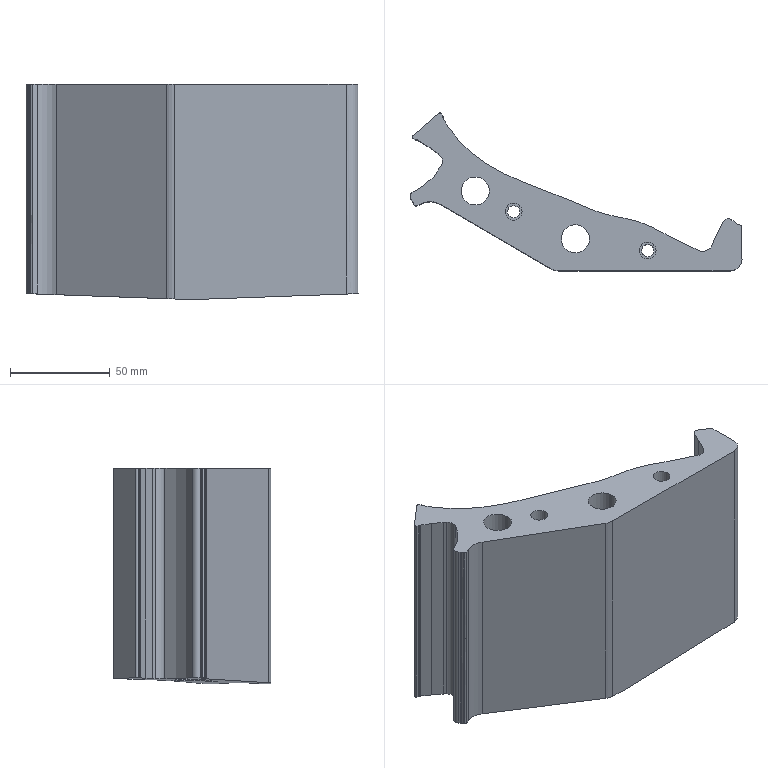Part | NX | features 8 2 | 1 solid | 62 faces | box 166.615 x 79.226 x 108 mm | volume 422130 mm3 | plane 26 | spline 22 | cylinder 14 | commonest cylinder face diameters 2 x4 20 x3 6.2 x2 8.5 x2 14.1 x2 16 x1